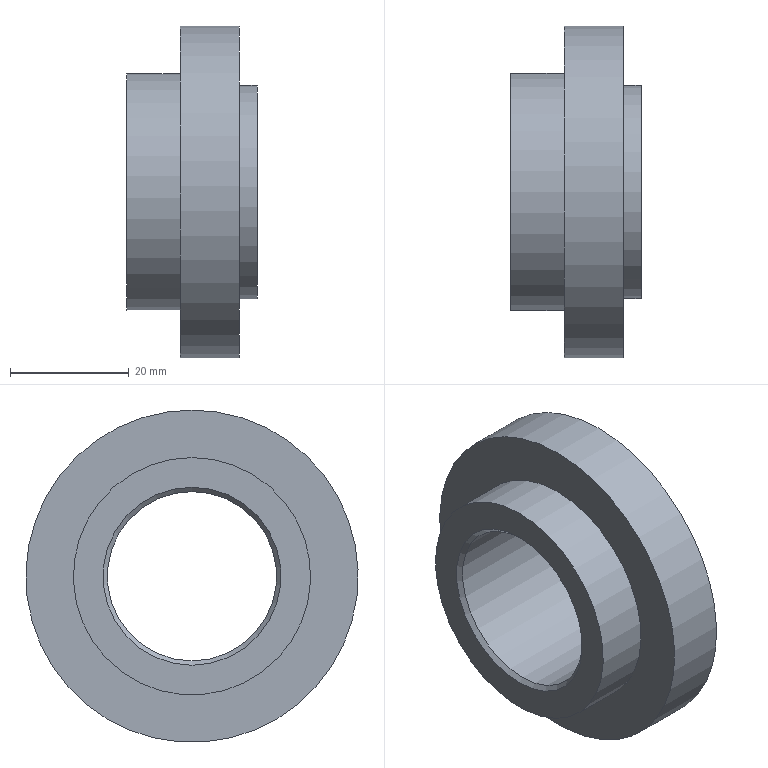Part | NX | features DATUM_CSYS 2, HOLE PACKAGE 1, SIMPLE HOLE 1, SKETCH 1, SWP104 1, SYMBOLIC_THREAD 1 | 1 solid | 10 faces | box 22 x 56 x 56 mm | volume 24872 mm3 | plane 4 | cylinder 4 | cone 2 | commonest cylinder face diameters 28.539 x1 36 x1 40 x1 56 x1
STEP:
#1=CARTESIAN_POINT('',(0.,0.,15.));
#2=VERTEX_POINT('',#1);
#3=CARTESIAN_POINT('',(0.,0.,0.));
#4=DIRECTION('',(-1.,0.,0.));
#5=DIRECTION('',(0.,0.,1.));
#6=AXIS2_PLACEMENT_3D('',#3,#4,#5);
#7=CIRCLE('',#6,15.);
#8=EDGE_CURVE('',#2,#2,#7,.F.);
#9=ORIENTED_EDGE('',*,*,#8,.T.);
#10=EDGE_LOOP('',(#9));
#11=FACE_BOUND('',#10,.T.);
#12=CARTESIAN_POINT('',(0.,0.,20.));
#13=VERTEX_POINT('',#12);
#14=CARTESIAN_POINT('',(0.,0.,0.));
#15=DIRECTION('',(-1.,0.,0.));
#16=DIRECTION('',(0.,0.,1.));
#17=AXIS2_PLACEMENT_3D('',#14,#15,#16);
#18=CIRCLE('',#17,20.);
#19=EDGE_CURVE('',#13,#13,#18,.T.);
#20=ORIENTED_EDGE('',*,*,#19,.T.);
#21=EDGE_LOOP('',(#20));
#22=FACE_BOUND('',#21,.T.);
#23=CARTESIAN_POINT('',(0.,0.,0.));
#24=DIRECTION('',(-1.,0.,0.));
#25=DIRECTION('',(0.,0.,1.));
#26=AXIS2_PLACEMENT_3D('',#23,#24,#25);
#27=PLANE('',#26);
#28=ADVANCED_FACE('',(#11,#22),#27,.T.);
#29=CARTESIAN_POINT('',(9.,0.,20.));
#30=VERTEX_POINT('',#29);
#31=CARTESIAN_POINT('',(9.,0.,0.));
#32=DIRECTION('',(-1.,0.,0.));
#33=DIRECTION('',(0.,0.,1.));
#34=AXIS2_PLACEMENT_3D('',#31,#32,#33);
#35=CIRCLE('',#34,20.);
#36=EDGE_CURVE('',#30,#30,#35,.T.);
#37=ORIENTED_EDGE('',*,*,#36,.T.);
#38=EDGE_LOOP('',(#37));
#39=FACE_BOUND('',#38,.T.);
#40=ORIENTED_EDGE('',*,*,#19,.F.);
#41=EDGE_LOOP('',(#40));
#42=FACE_BOUND('',#41,.T.);
#43=CARTESIAN_POINT('',(0.,0.,0.));
#44=DIRECTION('',(-1.,0.,0.));
#45=DIRECTION('',(0.,0.,1.));
#46=AXIS2_PLACEMENT_3D('',#43,#44,#45);
#47=CYLINDRICAL_SURFACE('',#46,20.);
#48=ADVANCED_FACE('',(#39,#42),#47,.T.);
#49=CARTESIAN_POINT('',(9.,0.,28.));
#50=VERTEX_POINT('',#49);
#51=CARTESIAN_POINT('',(9.,0.,0.));
#52=DIRECTION('',(-1.,0.,0.));
#53=DIRECTION('',(0.,0.,1.));
#54=AXIS2_PLACEMENT_3D('',#51,#52,#53);
#55=CIRCLE('',#54,28.);
#56=EDGE_CURVE('',#50,#50,#55,.T.);
#57=ORIENTED_EDGE('',*,*,#56,.T.);
#58=EDGE_LOOP('',(#57));
#59=FACE_BOUND('',#58,.T.);
#60=ORIENTED_EDGE('',*,*,#36,.F.);
#61=EDGE_LOOP('',(#60));
#62=FACE_BOUND('',#61,.T.);
#63=CARTESIAN_POINT('',(9.,20.,0.));
#64=DIRECTION('',(-1.,0.,0.));
#65=DIRECTION('',(0.,0.,1.));
#66=AXIS2_PLACEMENT_3D('',#63,#64,#65);
#67=PLANE('',#66);
#68=ADVANCED_FACE('',(#59,#62),#67,.T.);
#69=CARTESIAN_POINT('',(19.,0.,28.));
#70=VERTEX_POINT('',#69);
#71=CARTESIAN_POINT('',(19.,0.,0.));
#72=DIRECTION('',(-1.,0.,0.));
#73=DIRECTION('',(0.,0.,1.));
#74=AXIS2_PLACEMENT_3D('',#71,#72,#73);
#75=CIRCLE('',#74,28.);
#76=EDGE_CURVE('',#70,#70,#75,.T.);
#77=ORIENTED_EDGE('',*,*,#76,.T.);
#78=EDGE_LOOP('',(#77));
#79=FACE_BOUND('',#78,.T.);
#80=ORIENTED_EDGE('',*,*,#56,.F.);
#81=EDGE_LOOP('',(#80));
#82=FACE_BOUND('',#81,.T.);
#83=CARTESIAN_POINT('',(0.,0.,0.));
#84=DIRECTION('',(-1.,0.,0.));
#85=DIRECTION('',(0.,0.,1.));
#86=AXIS2_PLACEMENT_3D('',#83,#84,#85);
#87=CYLINDRICAL_SURFACE('',#86,28.);
#88=ADVANCED_FACE('',(#79,#82),#87,.T.);
#89=CARTESIAN_POINT('',(19.,0.,18.));
#90=VERTEX_POINT('',#89);
#91=CARTESIAN_POINT('',(19.,0.,0.));
#92=DIRECTION('',(-1.,0.,0.));
#93=DIRECTION('',(0.,0.,1.));
#94=AXIS2_PLACEMENT_3D('',#91,#92,#93);
#95=CIRCLE('',#94,18.);
#96=EDGE_CURVE('',#90,#90,#95,.T.);
#97=ORIENTED_EDGE('',*,*,#96,.T.);
#98=EDGE_LOOP('',(#97));
#99=FACE_BOUND('',#98,.T.);
#100=ORIENTED_EDGE('',*,*,#76,.F.);
#101=EDGE_LOOP('',(#100));
#102=FACE_BOUND('',#101,.T.);
#103=CARTESIAN_POINT('',(19.,28.,0.));
#104=DIRECTION('',(1.,0.,0.));
#105=DIRECTION('',(0.,0.,-1.));
#106=AXIS2_PLACEMENT_3D('',#103,#104,#105);
#107=PLANE('',#106);
#108=ADVANCED_FACE('',(#99,#102),#107,.T.);
#109=CARTESIAN_POINT('',(22.,0.,18.));
#110=VERTEX_POINT('',#109);
#111=CARTESIAN_POINT('',(22.,0.,0.));
#112=DIRECTION('',(-1.,0.,0.));
#113=DIRECTION('',(0.,0.,1.));
#114=AXIS2_PLACEMENT_3D('',#111,#112,#113);
#115=CIRCLE('',#114,18.);
#116=EDGE_CURVE('',#110,#110,#115,.T.);
#117=ORIENTED_EDGE('',*,*,#116,.T.);
#118=EDGE_LOOP('',(#117));
#119=FACE_BOUND('',#118,.T.);
#120=ORIENTED_EDGE('',*,*,#96,.F.);
#121=EDGE_LOOP('',(#120));
#122=FACE_BOUND('',#121,.T.);
#123=CARTESIAN_POINT('',(0.,0.,0.));
#124=DIRECTION('',(-1.,0.,0.));
#125=DIRECTION('',(0.,0.,1.));
#126=AXIS2_PLACEMENT_3D('',#123,#124,#125);
#127=CYLINDRICAL_SURFACE('',#126,18.);
#128=ADVANCED_FACE('',(#119,#122),#127,.T.);
#129=CARTESIAN_POINT('',(22.,0.,-15.));
#130=VERTEX_POINT('',#129);
#131=CARTESIAN_POINT('',(22.,0.,0.));
#132=DIRECTION('',(1.,0.,0.));
#133=DIRECTION('',(0.,0.,-1.));
#134=AXIS2_PLACEMENT_3D('',#131,#132,#133);
#135=CIRCLE('',#134,15.);
#136=EDGE_CURVE('',#130,#130,#135,.F.);
#137=ORIENTED_EDGE('',*,*,#136,.T.);
#138=EDGE_LOOP('',(#137));
#139=FACE_BOUND('',#138,.T.);
#140=ORIENTED_EDGE('',*,*,#116,.F.);
#141=EDGE_LOOP('',(#140));
#142=FACE_BOUND('',#141,.T.);
#143=CARTESIAN_POINT('',(22.,18.,0.));
#144=DIRECTION('',(1.,0.,0.));
#145=DIRECTION('',(0.,0.,-1.));
#146=AXIS2_PLACEMENT_3D('',#143,#144,#145);
#147=PLANE('',#146);
#148=ADVANCED_FACE('',(#139,#142),#147,.T.);
#149=CARTESIAN_POINT('',(21.27,0.,-14.27));
#150=VERTEX_POINT('',#149);
#151=CARTESIAN_POINT('',(21.27,0.,0.));
#152=DIRECTION('',(1.,0.,0.));
#153=DIRECTION('',(0.,0.,-1.));
#154=AXIS2_PLACEMENT_3D('',#151,#152,#153);
#155=CIRCLE('',#154,14.27);
#156=EDGE_CURVE('',#150,#150,#155,.T.);
#157=ORIENTED_EDGE('',*,*,#156,.T.);
#158=EDGE_LOOP('',(#157));
#159=FACE_BOUND('',#158,.T.);
#160=CARTESIAN_POINT('',(0.7305,0.,14.27));
#161=VERTEX_POINT('',#160);
#162=CARTESIAN_POINT('',(0.7305,0.,0.));
#163=DIRECTION('',(-1.,0.,0.));
#164=DIRECTION('',(0.,0.,1.));
#165=AXIS2_PLACEMENT_3D('',#162,#163,#164);
#166=CIRCLE('',#165,14.27);
#167=EDGE_CURVE('',#161,#161,#166,.T.);
#168=ORIENTED_EDGE('',*,*,#167,.T.);
#169=EDGE_LOOP('',(#168));
#170=FACE_BOUND('',#169,.T.);
#171=CARTESIAN_POINT('',(0.,0.,0.));
#172=DIRECTION('',(1.,0.,0.));
#173=DIRECTION('',(0.,0.,-1.));
#174=AXIS2_PLACEMENT_3D('',#171,#172,#173);
#175=CYLINDRICAL_SURFACE('',#174,14.27);
#176=ADVANCED_FACE('',(#159,#170),#175,.F.);
#177=ORIENTED_EDGE('',*,*,#167,.F.);
#178=EDGE_LOOP('',(#177));
#179=FACE_BOUND('',#178,.T.);
#180=ORIENTED_EDGE('',*,*,#8,.F.);
#181=EDGE_LOOP('',(#180));
#182=FACE_BOUND('',#181,.T.);
#183=CARTESIAN_POINT('',(0.,0.,0.));
#184=DIRECTION('',(-1.,0.,0.));
#185=DIRECTION('',(0.,0.,1.));
#186=AXIS2_PLACEMENT_3D('',#183,#184,#185);
#187=CONICAL_SURFACE('',#186,15.,0.7854);
#188=ADVANCED_FACE('',(#179,#182),#187,.F.);
#189=ORIENTED_EDGE('',*,*,#136,.F.);
#190=EDGE_LOOP('',(#189));
#191=FACE_BOUND('',#190,.T.);
#192=ORIENTED_EDGE('',*,*,#156,.F.);
#193=EDGE_LOOP('',(#192));
#194=FACE_BOUND('',#193,.T.);
#195=CARTESIAN_POINT('',(21.27,0.,0.));
#196=DIRECTION('',(1.,0.,0.));
#197=DIRECTION('',(0.,0.,-1.));
#198=AXIS2_PLACEMENT_3D('',#195,#196,#197);
#199=CONICAL_SURFACE('',#198,14.27,0.7854);
#200=ADVANCED_FACE('',(#191,#194),#199,.F.);
#201=CLOSED_SHELL('',(#28,#48,#68,#88,#108,#128,#148,#176,#188,#200));
#202=MANIFOLD_SOLID_BREP('',#201);
#203=(LENGTH_UNIT()NAMED_UNIT(*)SI_UNIT(.MILLI.,.METRE.));
#204=UNCERTAINTY_MEASURE_WITH_UNIT(LENGTH_MEASURE(0.00001),#203,'','');
#205=(NAMED_UNIT(*)PLANE_ANGLE_UNIT()SI_UNIT($,.RADIAN.));
#206=(NAMED_UNIT(*)SI_UNIT($,.STERADIAN.)SOLID_ANGLE_UNIT());
#207=(GEOMETRIC_REPRESENTATION_CONTEXT(3)GLOBAL_UNCERTAINTY_ASSIGNED_CONTEXT((#204))GLOBAL_UNIT_ASSIGNED_CONTEXT((#203,#205,#206))REPRESENTATION_CONTEXT('',''));
#208=ADVANCED_BREP_SHAPE_REPRESENTATION('',(#202),#207);